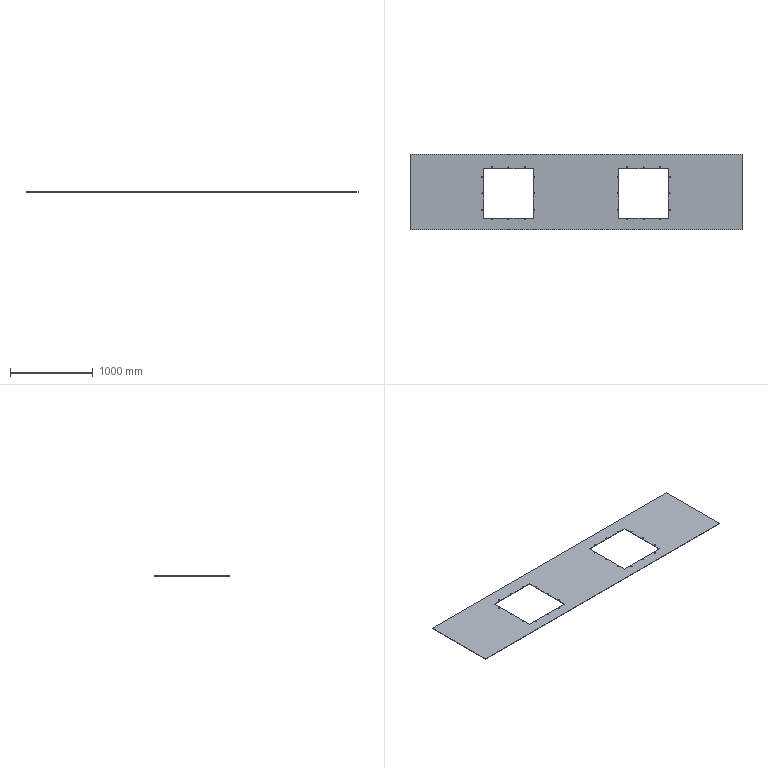Part | SolidWorks | features ICE 2, FlatPattern 1, LPattern 1, SMBaseFlange 1, SheetMetal 1 | 1 solid | 62 faces | box 4020 x 910 x 5 mm | volume 14675072 mm3 | cylinder 48 | plane 14 | commonest cylinder face diameters 13 x48